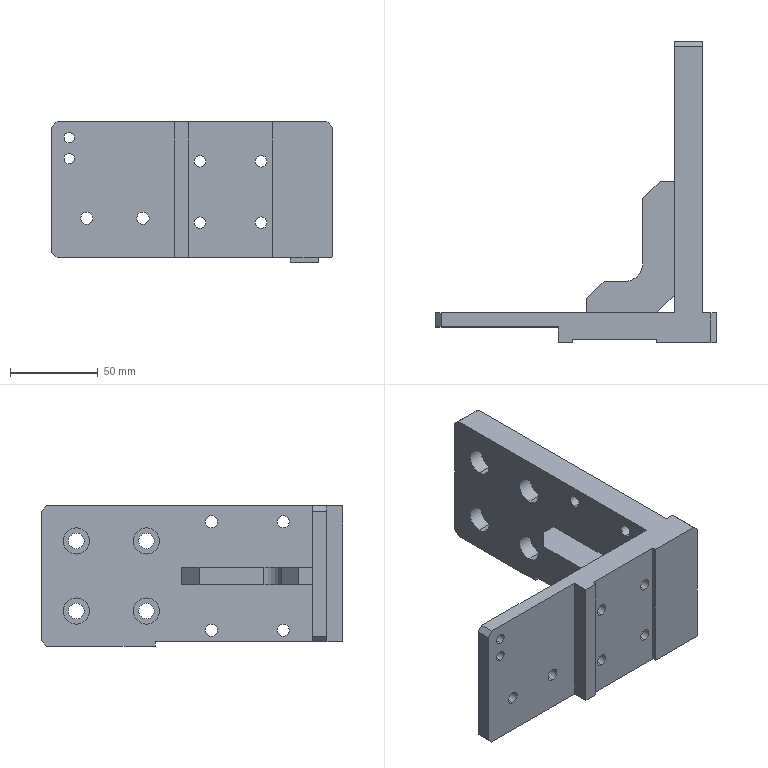Part | SolidWorks | features HoleWzd 7, ICE 4, Chamfer 3, Extrusion 1, Fillet 1 | 1 solid | 90 faces | box 160 x 172 x 80 mm | volume 351912 mm3 | cylinder 49 | plane 41 | commonest cylinder face diameters 7 x12 6.6 x8 9 x8 11 x8 15 x8 6 x4